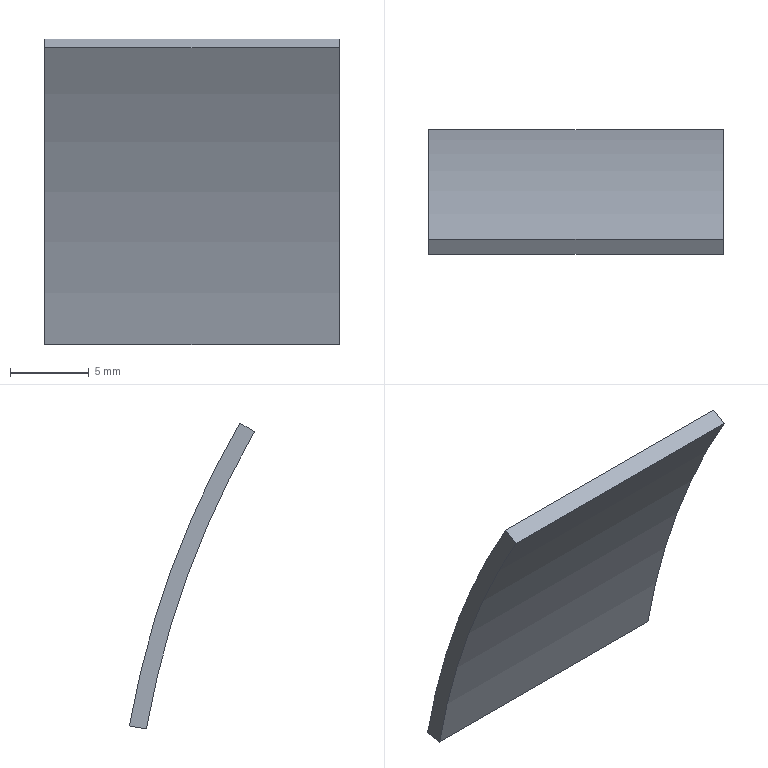Part | STEP file | basic_gh_motor_gh1_15 | 1 solid | 6 faces | box 18.75 x 7.973 x 19.478 mm | volume 421.53 mm3 | plane 4 | cylinder 2 | commonest cylinder face diameters 116 x1 118.2 x1
STEP:
#1=CARTESIAN_POINT('',(-90.,130.702,10.263));
#2=VERTEX_POINT('',#1);
#3=CARTESIAN_POINT('',(-90.,123.682,29.55));
#4=VERTEX_POINT('',#3);
#5=CARTESIAN_POINT('',(-90.,72.5,0.));
#6=DIRECTION('',(1.,0.,0.));
#7=DIRECTION('',(0.,0.,1.));
#8=AXIS2_PLACEMENT_3D('',#5,#6,#7);
#9=CIRCLE('',#8,59.1);
#10=EDGE_CURVE('',#2,#4,#9,.T.);
#11=ORIENTED_EDGE('',*,*,#10,.T.);
#12=CARTESIAN_POINT('',(-71.25,123.682,29.55));
#13=VERTEX_POINT('',#12);
#14=CARTESIAN_POINT('',(-71.25,123.682,29.55));
#15=DIRECTION('',(-1.,0.,0.));
#16=VECTOR('',#15,1.);
#17=LINE('',#14,#16);
#18=EDGE_CURVE('',#13,#4,#17,.T.);
#19=ORIENTED_EDGE('',*,*,#18,.F.);
#20=CARTESIAN_POINT('',(-71.25,130.702,10.263));
#21=VERTEX_POINT('',#20);
#22=CARTESIAN_POINT('',(-71.25,72.5,0.));
#23=DIRECTION('',(-1.,0.,0.));
#24=DIRECTION('',(0.,0.,1.));
#25=AXIS2_PLACEMENT_3D('',#22,#23,#24);
#26=CIRCLE('',#25,59.1);
#27=EDGE_CURVE('',#13,#21,#26,.T.);
#28=ORIENTED_EDGE('',*,*,#27,.T.);
#29=CARTESIAN_POINT('',(-71.25,130.702,10.263));
#30=DIRECTION('',(-1.,0.,0.));
#31=VECTOR('',#30,1.);
#32=LINE('',#29,#31);
#33=EDGE_CURVE('',#21,#2,#32,.T.);
#34=ORIENTED_EDGE('',*,*,#33,.T.);
#35=EDGE_LOOP('',(#11,#19,#28,#34));
#36=FACE_OUTER_BOUND('',#35,.T.);
#37=CARTESIAN_POINT('',(-71.25,72.5,0.));
#38=DIRECTION('',(-1.,0.,0.));
#39=DIRECTION('',(0.,0.,1.));
#40=AXIS2_PLACEMENT_3D('',#37,#38,#39);
#41=CYLINDRICAL_SURFACE('',#40,59.1);
#42=ADVANCED_FACE('',(#36),#41,.T.);
#43=CARTESIAN_POINT('',(-90.,122.729,29.));
#44=VERTEX_POINT('',#43);
#45=CARTESIAN_POINT('',(-90.,122.729,29.));
#46=DIRECTION('',(0.,-0.866,-0.5));
#47=VECTOR('',#46,1.);
#48=LINE('',#45,#47);
#49=EDGE_CURVE('',#4,#44,#48,.T.);
#50=ORIENTED_EDGE('',*,*,#49,.T.);
#51=CARTESIAN_POINT('',(-71.25,122.729,29.));
#52=VERTEX_POINT('',#51);
#53=CARTESIAN_POINT('',(-71.25,122.729,29.));
#54=DIRECTION('',(-1.,0.,0.));
#55=VECTOR('',#54,1.);
#56=LINE('',#53,#55);
#57=EDGE_CURVE('',#52,#44,#56,.T.);
#58=ORIENTED_EDGE('',*,*,#57,.F.);
#59=CARTESIAN_POINT('',(-71.25,122.729,29.));
#60=DIRECTION('',(0.,0.866,0.5));
#61=VECTOR('',#60,1.);
#62=LINE('',#59,#61);
#63=EDGE_CURVE('',#52,#13,#62,.T.);
#64=ORIENTED_EDGE('',*,*,#63,.T.);
#65=ORIENTED_EDGE('',*,*,#18,.T.);
#66=EDGE_LOOP('',(#50,#58,#64,#65));
#67=FACE_OUTER_BOUND('',#66,.T.);
#68=CARTESIAN_POINT('',(-71.25,123.206,29.275));
#69=DIRECTION('',(0.,-0.5,0.866));
#70=DIRECTION('',(0.,0.866,0.5));
#71=AXIS2_PLACEMENT_3D('',#68,#69,#70);
#72=PLANE('',#71);
#73=ADVANCED_FACE('',(#67),#72,.T.);
#74=CARTESIAN_POINT('',(-90.,129.619,10.072));
#75=VERTEX_POINT('',#74);
#76=CARTESIAN_POINT('',(-90.,72.5,0.));
#77=DIRECTION('',(-1.,0.,0.));
#78=DIRECTION('',(0.,0.,1.));
#79=AXIS2_PLACEMENT_3D('',#76,#77,#78);
#80=CIRCLE('',#79,58.);
#81=EDGE_CURVE('',#44,#75,#80,.T.);
#82=ORIENTED_EDGE('',*,*,#81,.T.);
#83=CARTESIAN_POINT('',(-71.25,129.619,10.072));
#84=VERTEX_POINT('',#83);
#85=CARTESIAN_POINT('',(-71.25,129.619,10.072));
#86=DIRECTION('',(-1.,0.,0.));
#87=VECTOR('',#86,1.);
#88=LINE('',#85,#87);
#89=EDGE_CURVE('',#84,#75,#88,.T.);
#90=ORIENTED_EDGE('',*,*,#89,.F.);
#91=CARTESIAN_POINT('',(-71.25,72.5,0.));
#92=DIRECTION('',(-1.,0.,0.));
#93=DIRECTION('',(0.,0.,1.));
#94=AXIS2_PLACEMENT_3D('',#91,#92,#93);
#95=CIRCLE('',#94,58.);
#96=EDGE_CURVE('',#52,#84,#95,.T.);
#97=ORIENTED_EDGE('',*,*,#96,.F.);
#98=ORIENTED_EDGE('',*,*,#57,.T.);
#99=EDGE_LOOP('',(#82,#90,#97,#98));
#100=FACE_OUTER_BOUND('',#99,.T.);
#101=CARTESIAN_POINT('',(-71.25,72.5,0.));
#102=DIRECTION('',(-1.,0.,0.));
#103=DIRECTION('',(0.,0.,1.));
#104=AXIS2_PLACEMENT_3D('',#101,#102,#103);
#105=CYLINDRICAL_SURFACE('',#104,58.);
#106=ADVANCED_FACE('',(#100),#105,.F.);
#107=CARTESIAN_POINT('',(-90.,129.619,10.072));
#108=DIRECTION('',(0.,0.9848,0.1736));
#109=VECTOR('',#108,1.);
#110=LINE('',#107,#109);
#111=EDGE_CURVE('',#75,#2,#110,.T.);
#112=ORIENTED_EDGE('',*,*,#111,.T.);
#113=ORIENTED_EDGE('',*,*,#33,.F.);
#114=CARTESIAN_POINT('',(-71.25,129.619,10.072));
#115=DIRECTION('',(0.,0.9848,0.1736));
#116=VECTOR('',#115,1.);
#117=LINE('',#114,#116);
#118=EDGE_CURVE('',#84,#21,#117,.T.);
#119=ORIENTED_EDGE('',*,*,#118,.F.);
#120=ORIENTED_EDGE('',*,*,#89,.T.);
#121=EDGE_LOOP('',(#112,#113,#119,#120));
#122=FACE_OUTER_BOUND('',#121,.T.);
#123=CARTESIAN_POINT('',(-71.25,130.16,10.167));
#124=DIRECTION('',(0.,0.1736,-0.9848));
#125=DIRECTION('',(0.,-0.9848,-0.1736));
#126=AXIS2_PLACEMENT_3D('',#123,#124,#125);
#127=PLANE('',#126);
#128=ADVANCED_FACE('',(#122),#127,.T.);
#129=ORIENTED_EDGE('',*,*,#10,.F.);
#130=ORIENTED_EDGE('',*,*,#111,.F.);
#131=ORIENTED_EDGE('',*,*,#81,.F.);
#132=ORIENTED_EDGE('',*,*,#49,.F.);
#133=EDGE_LOOP('',(#129,#130,#131,#132));
#134=FACE_OUTER_BOUND('',#133,.T.);
#135=CARTESIAN_POINT('',(-90.,127.163,19.896));
#136=DIRECTION('',(-1.,0.,0.));
#137=DIRECTION('',(0.,0.,1.));
#138=AXIS2_PLACEMENT_3D('',#135,#136,#137);
#139=PLANE('',#138);
#140=ADVANCED_FACE('',(#134),#139,.T.);
#141=ORIENTED_EDGE('',*,*,#118,.T.);
#142=ORIENTED_EDGE('',*,*,#27,.F.);
#143=ORIENTED_EDGE('',*,*,#63,.F.);
#144=ORIENTED_EDGE('',*,*,#96,.T.);
#145=EDGE_LOOP('',(#141,#142,#143,#144));
#146=FACE_OUTER_BOUND('',#145,.T.);
#147=CARTESIAN_POINT('',(-71.25,127.163,19.896));
#148=DIRECTION('',(-1.,0.,0.));
#149=DIRECTION('',(0.,0.,1.));
#150=AXIS2_PLACEMENT_3D('',#147,#148,#149);
#151=PLANE('',#150);
#152=ADVANCED_FACE('',(#146),#151,.F.);
#153=CLOSED_SHELL('',(#42,#73,#106,#128,#140,#152));
#154=MANIFOLD_SOLID_BREP('',#153);
#155=(LENGTH_UNIT()NAMED_UNIT(*)SI_UNIT(.MILLI.,.METRE.));
#156=UNCERTAINTY_MEASURE_WITH_UNIT(LENGTH_MEASURE(0.01),#155,'','');
#157=(NAMED_UNIT(*)PLANE_ANGLE_UNIT()SI_UNIT($,.RADIAN.));
#158=(NAMED_UNIT(*)SI_UNIT($,.STERADIAN.)SOLID_ANGLE_UNIT());
#159=(GEOMETRIC_REPRESENTATION_CONTEXT(3)GLOBAL_UNCERTAINTY_ASSIGNED_CONTEXT((#156))GLOBAL_UNIT_ASSIGNED_CONTEXT((#155,#157,#158))REPRESENTATION_CONTEXT('',''));
#160=ADVANCED_BREP_SHAPE_REPRESENTATION('',(#154),#159);